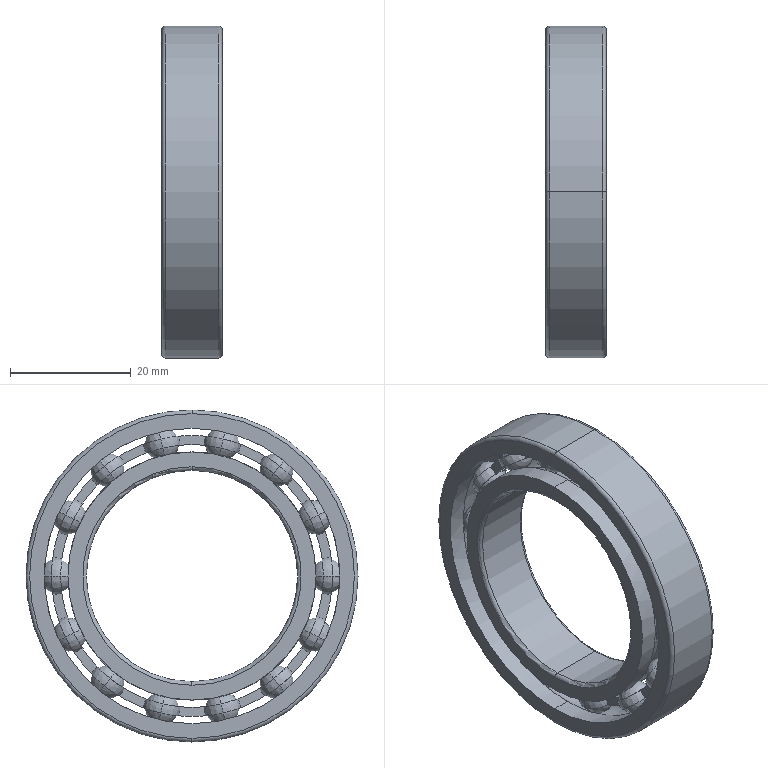Part | SolidWorks | features Revolution 5, CirPattern 2, RevCut 2 | 1 solid | 213 faces | box 10 x 55 x 55 mm | volume 9427 mm3 | sphere 112 | torus 53 | plane 32 | cylinder 16 | commonest cylinder face diameters 41.1 x4 48.9 x4 35 x2 43.472 x2 46.528 x2 55 x2